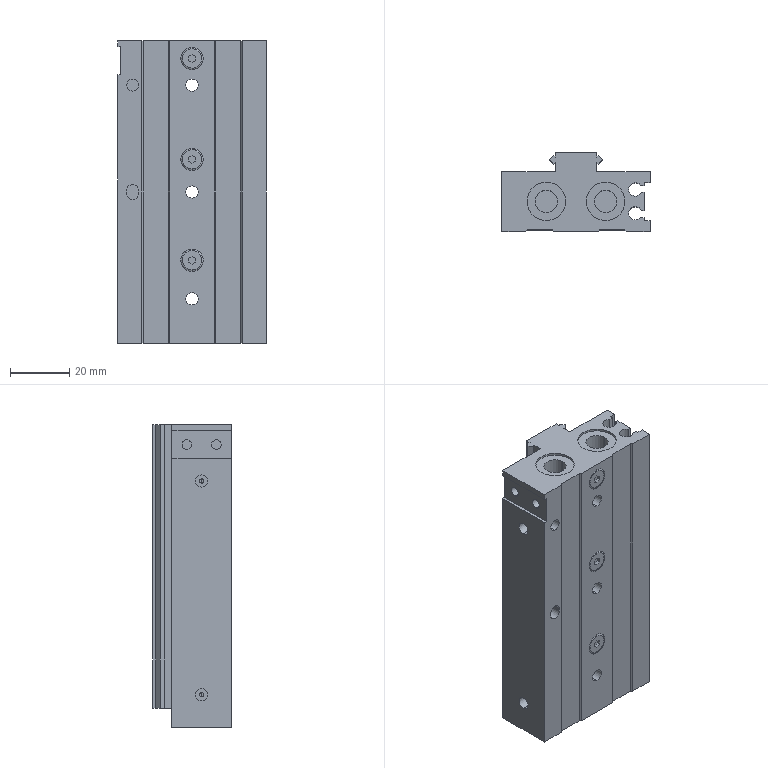Part | STEP file | QA-HI_MDX12x50-SD2BM2(0)_Bo | 1 solid | 162 faces | box 50 x 26.5 x 102 mm | volume 80346 mm3 | plane 93 | cylinder 63 | spline 6 | commonest cylinder face diameters 3.242 x12 4.134 x10 7.5 x10 13 x8 8.5 x6 4 x5